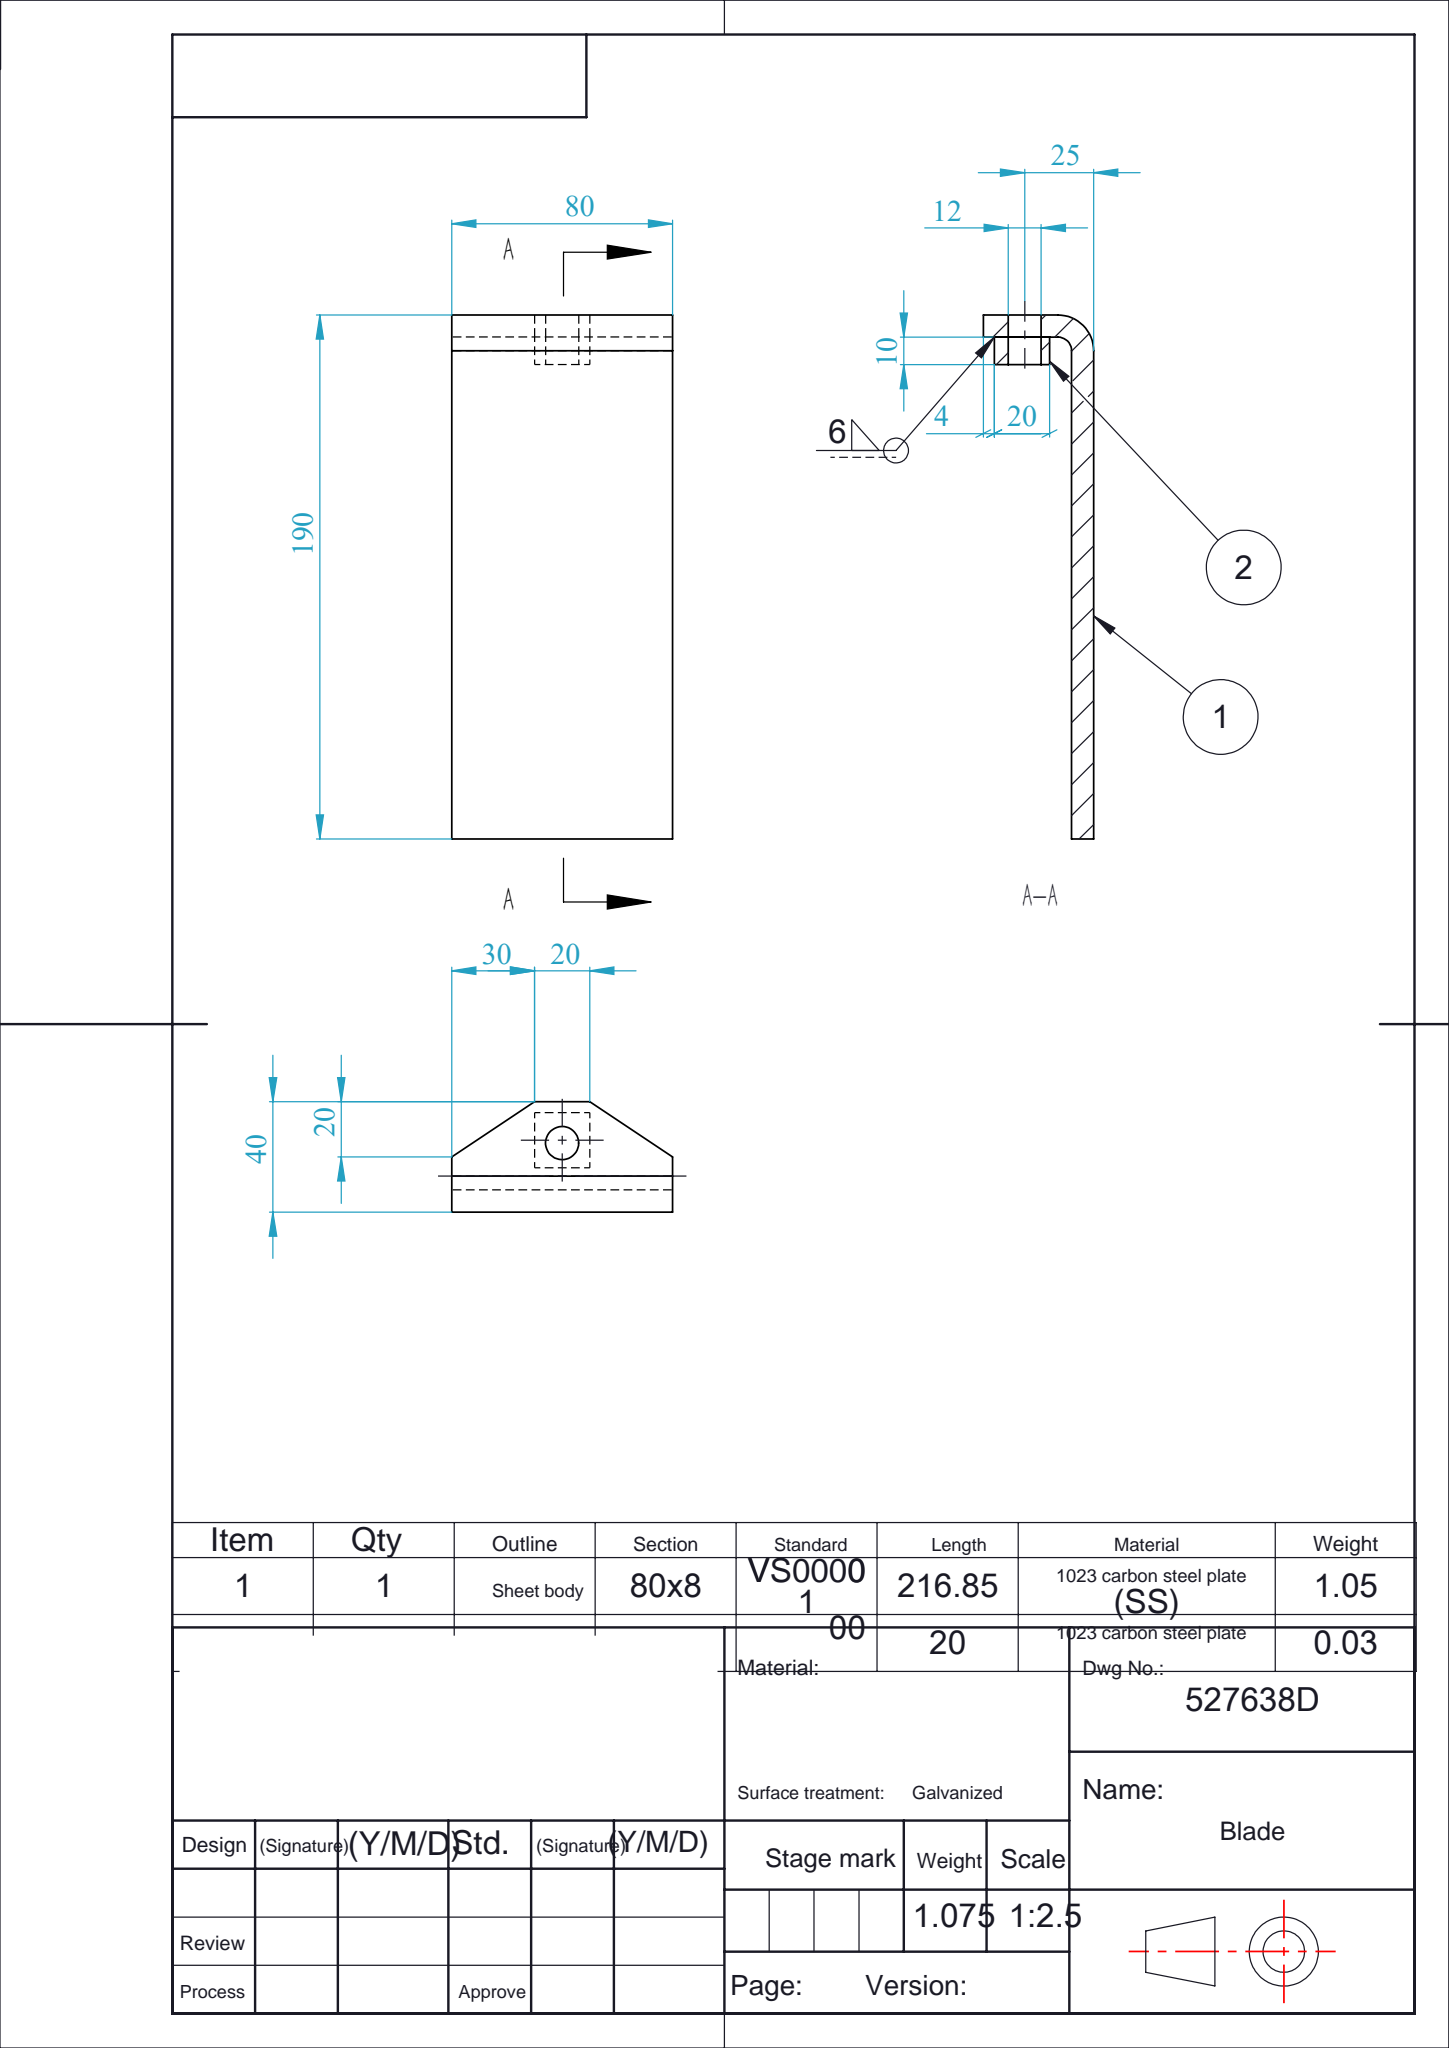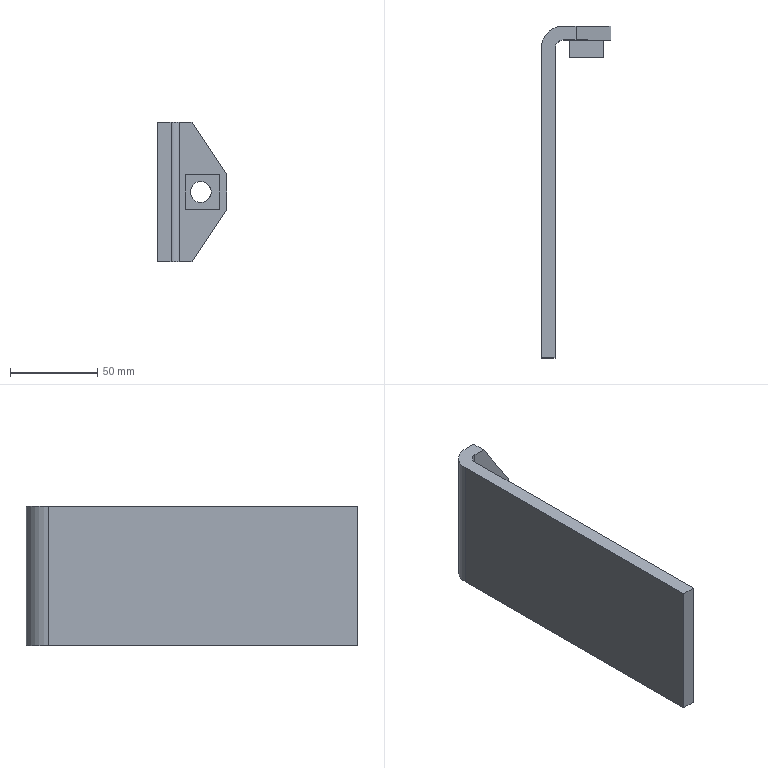Part | SolidWorks | features CompositeCurve 1 | 2 solids | 22 faces | box 40 x 190 x 80 mm | volume 136772 mm3 | plane 16 | cylinder 6 | commonest cylinder face diameters 12 x4 10 x1 26 x1